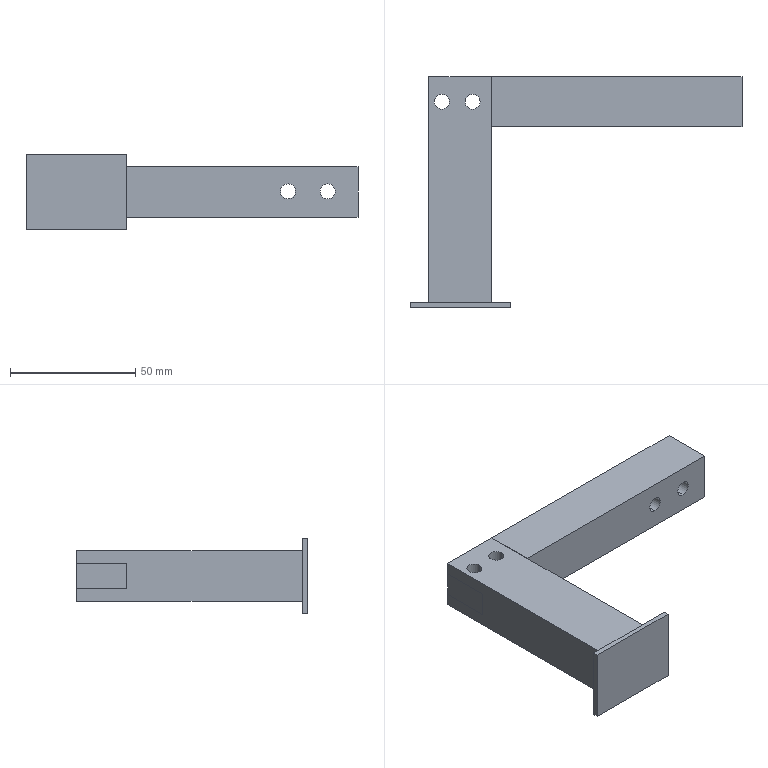Part | SolidWorks | features Cut 3, ICE 2, Extrusion 1 | 2 solids | 41 faces | box 132.5 x 92 x 30 mm | volume 85138 mm3 | plane 25 | cylinder 16 | commonest cylinder face diameters 6 x16
STEP:
#1=CARTESIAN_POINT('',(-15.29,82.,4.756));
#2=VERTEX_POINT('',#1);
#3=CARTESIAN_POINT('',(-9.29,82.,4.756));
#4=VERTEX_POINT('',#3);
#5=CARTESIAN_POINT('',(-12.29,82.,4.756));
#6=DIRECTION('',(0.,0.,1.));
#7=DIRECTION('',(1.,0.,0.));
#8=AXIS2_PLACEMENT_3D('',#5,#6,#7);
#9=CIRCLE('',#8,3.);
#10=EDGE_CURVE('',#2,#4,#9,.T.);
#11=ORIENTED_EDGE('',*,*,#10,.F.);
#12=CARTESIAN_POINT('',(-15.29,82.,9.756));
#13=VERTEX_POINT('',#12);
#14=CARTESIAN_POINT('',(-15.29,82.,-19.244));
#15=DIRECTION('',(0.,0.,1.));
#16=VECTOR('',#15,1000.);
#17=LINE('',#14,#16);
#18=EDGE_CURVE('',#2,#13,#17,.T.);
#19=ORIENTED_EDGE('',*,*,#18,.T.);
#20=CARTESIAN_POINT('',(-9.29,82.,9.756));
#21=VERTEX_POINT('',#20);
#22=CARTESIAN_POINT('',(-12.29,82.,9.756));
#23=DIRECTION('',(0.,0.,1.));
#24=DIRECTION('',(1.,0.,0.));
#25=AXIS2_PLACEMENT_3D('',#22,#23,#24);
#26=CIRCLE('',#25,3.);
#27=EDGE_CURVE('',#13,#21,#26,.T.);
#28=ORIENTED_EDGE('',*,*,#27,.T.);
#29=CARTESIAN_POINT('',(-9.29,82.,-19.244));
#30=DIRECTION('',(0.,0.,1.));
#31=VECTOR('',#30,1000.);
#32=LINE('',#29,#31);
#33=EDGE_CURVE('',#4,#21,#32,.T.);
#34=ORIENTED_EDGE('',*,*,#33,.F.);
#35=EDGE_LOOP('',(#11,#19,#28,#34));
#36=FACE_OUTER_BOUND('',#35,.T.);
#37=CARTESIAN_POINT('',(-12.29,82.,-19.244));
#38=DIRECTION('',(0.,0.,1.));
#39=DIRECTION('',(1.,0.,0.));
#40=AXIS2_PLACEMENT_3D('',#37,#38,#39);
#41=CYLINDRICAL_SURFACE('',#40,3.);
#42=ADVANCED_FACE('',(#36),#41,.F.);
#43=CARTESIAN_POINT('',(-3.,82.,4.756));
#44=VERTEX_POINT('',#43);
#45=CARTESIAN_POINT('',(3.,82.,4.756));
#46=VERTEX_POINT('',#45);
#47=CARTESIAN_POINT('',(0.,82.,4.756));
#48=DIRECTION('',(0.,0.,1.));
#49=DIRECTION('',(1.,0.,0.));
#50=AXIS2_PLACEMENT_3D('',#47,#48,#49);
#51=CIRCLE('',#50,3.);
#52=EDGE_CURVE('',#44,#46,#51,.T.);
#53=ORIENTED_EDGE('',*,*,#52,.F.);
#54=CARTESIAN_POINT('',(-3.,82.,9.756));
#55=VERTEX_POINT('',#54);
#56=CARTESIAN_POINT('',(-3.,82.,-19.244));
#57=DIRECTION('',(0.,0.,1.));
#58=VECTOR('',#57,1000.);
#59=LINE('',#56,#58);
#60=EDGE_CURVE('',#44,#55,#59,.T.);
#61=ORIENTED_EDGE('',*,*,#60,.T.);
#62=CARTESIAN_POINT('',(3.,82.,9.756));
#63=VERTEX_POINT('',#62);
#64=CARTESIAN_POINT('',(0.,82.,9.756));
#65=DIRECTION('',(0.,0.,1.));
#66=DIRECTION('',(1.,0.,0.));
#67=AXIS2_PLACEMENT_3D('',#64,#65,#66);
#68=CIRCLE('',#67,3.);
#69=EDGE_CURVE('',#55,#63,#68,.T.);
#70=ORIENTED_EDGE('',*,*,#69,.T.);
#71=CARTESIAN_POINT('',(3.,82.,-19.244));
#72=DIRECTION('',(0.,0.,1.));
#73=VECTOR('',#72,1000.);
#74=LINE('',#71,#73);
#75=EDGE_CURVE('',#46,#63,#74,.T.);
#76=ORIENTED_EDGE('',*,*,#75,.F.);
#77=EDGE_LOOP('',(#53,#61,#70,#76));
#78=FACE_OUTER_BOUND('',#77,.T.);
#79=CARTESIAN_POINT('',(0.,82.,-19.244));
#80=DIRECTION('',(0.,0.,1.));
#81=DIRECTION('',(1.,0.,0.));
#82=AXIS2_PLACEMENT_3D('',#79,#80,#81);
#83=CYLINDRICAL_SURFACE('',#82,3.);
#84=ADVANCED_FACE('',(#78),#83,.F.);
#85=CARTESIAN_POINT('',(-15.29,82.,-10.244));
#86=VERTEX_POINT('',#85);
#87=CARTESIAN_POINT('',(-9.29,82.,-10.244));
#88=VERTEX_POINT('',#87);
#89=CARTESIAN_POINT('',(-12.29,82.,-10.244));
#90=DIRECTION('',(0.,0.,1.));
#91=DIRECTION('',(1.,0.,0.));
#92=AXIS2_PLACEMENT_3D('',#89,#90,#91);
#93=CIRCLE('',#92,3.);
#94=EDGE_CURVE('',#86,#88,#93,.T.);
#95=ORIENTED_EDGE('',*,*,#94,.F.);
#96=CARTESIAN_POINT('',(-15.29,82.,-5.244));
#97=VERTEX_POINT('',#96);
#98=CARTESIAN_POINT('',(-15.29,82.,-19.244));
#99=DIRECTION('',(0.,0.,1.));
#100=VECTOR('',#99,1000.);
#101=LINE('',#98,#100);
#102=EDGE_CURVE('',#86,#97,#101,.T.);
#103=ORIENTED_EDGE('',*,*,#102,.T.);
#104=CARTESIAN_POINT('',(-9.29,82.,-5.244));
#105=VERTEX_POINT('',#104);
#106=CARTESIAN_POINT('',(-12.29,82.,-5.244));
#107=DIRECTION('',(0.,0.,-1.));
#108=DIRECTION('',(-1.,0.,0.));
#109=AXIS2_PLACEMENT_3D('',#106,#107,#108);
#110=CIRCLE('',#109,3.);
#111=EDGE_CURVE('',#105,#97,#110,.T.);
#112=ORIENTED_EDGE('',*,*,#111,.F.);
#113=CARTESIAN_POINT('',(-9.29,82.,-19.244));
#114=DIRECTION('',(0.,0.,1.));
#115=VECTOR('',#114,1000.);
#116=LINE('',#113,#115);
#117=EDGE_CURVE('',#88,#105,#116,.T.);
#118=ORIENTED_EDGE('',*,*,#117,.F.);
#119=EDGE_LOOP('',(#95,#103,#112,#118));
#120=FACE_OUTER_BOUND('',#119,.T.);
#121=CARTESIAN_POINT('',(-12.29,82.,-19.244));
#122=DIRECTION('',(0.,0.,1.));
#123=DIRECTION('',(1.,0.,0.));
#124=AXIS2_PLACEMENT_3D('',#121,#122,#123);
#125=CYLINDRICAL_SURFACE('',#124,3.);
#126=ADVANCED_FACE('',(#120),#125,.F.);
#127=CARTESIAN_POINT('',(-3.,82.,-10.244));
#128=VERTEX_POINT('',#127);
#129=CARTESIAN_POINT('',(3.,82.,-10.244));
#130=VERTEX_POINT('',#129);
#131=CARTESIAN_POINT('',(0.,82.,-10.244));
#132=DIRECTION('',(0.,0.,1.));
#133=DIRECTION('',(1.,0.,0.));
#134=AXIS2_PLACEMENT_3D('',#131,#132,#133);
#135=CIRCLE('',#134,3.);
#136=EDGE_CURVE('',#128,#130,#135,.T.);
#137=ORIENTED_EDGE('',*,*,#136,.F.);
#138=CARTESIAN_POINT('',(-3.,82.,-5.244));
#139=VERTEX_POINT('',#138);
#140=CARTESIAN_POINT('',(-3.,82.,-19.244));
#141=DIRECTION('',(0.,0.,1.));
#142=VECTOR('',#141,1000.);
#143=LINE('',#140,#142);
#144=EDGE_CURVE('',#128,#139,#143,.T.);
#145=ORIENTED_EDGE('',*,*,#144,.T.);
#146=CARTESIAN_POINT('',(3.,82.,-5.244));
#147=VERTEX_POINT('',#146);
#148=CARTESIAN_POINT('',(0.,82.,-5.244));
#149=DIRECTION('',(0.,0.,-1.));
#150=DIRECTION('',(-1.,0.,0.));
#151=AXIS2_PLACEMENT_3D('',#148,#149,#150);
#152=CIRCLE('',#151,3.);
#153=EDGE_CURVE('',#147,#139,#152,.T.);
#154=ORIENTED_EDGE('',*,*,#153,.F.);
#155=CARTESIAN_POINT('',(3.,82.,-19.244));
#156=DIRECTION('',(0.,0.,1.));
#157=VECTOR('',#156,1000.);
#158=LINE('',#155,#157);
#159=EDGE_CURVE('',#130,#147,#158,.T.);
#160=ORIENTED_EDGE('',*,*,#159,.F.);
#161=EDGE_LOOP('',(#137,#145,#154,#160));
#162=FACE_OUTER_BOUND('',#161,.T.);
#163=CARTESIAN_POINT('',(0.,82.,-19.244));
#164=DIRECTION('',(0.,0.,1.));
#165=DIRECTION('',(1.,0.,0.));
#166=AXIS2_PLACEMENT_3D('',#163,#164,#165);
#167=CYLINDRICAL_SURFACE('',#166,3.);
#168=ADVANCED_FACE('',(#162),#167,.F.);
#169=CARTESIAN_POINT('',(-17.5,92.,4.756));
#170=VERTEX_POINT('',#169);
#171=CARTESIAN_POINT('',(7.5,92.,4.756));
#172=VERTEX_POINT('',#171);
#173=CARTESIAN_POINT('',(-17.5,92.,4.756));
#174=DIRECTION('',(1.,0.,0.));
#175=VECTOR('',#174,1000.);
#176=LINE('',#173,#175);
#177=EDGE_CURVE('',#170,#172,#176,.T.);
#178=ORIENTED_EDGE('',*,*,#177,.F.);
#179=CARTESIAN_POINT('',(-17.5,92.,9.756));
#180=VERTEX_POINT('',#179);
#181=CARTESIAN_POINT('',(-17.5,92.,-10.244));
#182=DIRECTION('',(0.,0.,1.));
#183=VECTOR('',#182,1000.);
#184=LINE('',#181,#183);
#185=EDGE_CURVE('',#170,#180,#184,.T.);
#186=ORIENTED_EDGE('',*,*,#185,.T.);
#187=CARTESIAN_POINT('',(7.5,92.,9.756));
#188=VERTEX_POINT('',#187);
#189=CARTESIAN_POINT('',(-17.5,92.,9.756));
#190=DIRECTION('',(1.,0.,0.));
#191=VECTOR('',#190,1000.);
#192=LINE('',#189,#191);
#193=EDGE_CURVE('',#180,#188,#192,.T.);
#194=ORIENTED_EDGE('',*,*,#193,.T.);
#195=CARTESIAN_POINT('',(7.5,92.,-10.244));
#196=DIRECTION('',(0.,0.,-1.));
#197=VECTOR('',#196,1000.);
#198=LINE('',#195,#197);
#199=EDGE_CURVE('',#188,#172,#198,.T.);
#200=ORIENTED_EDGE('',*,*,#199,.T.);
#201=EDGE_LOOP('',(#178,#186,#194,#200));
#202=FACE_OUTER_BOUND('',#201,.T.);
#203=CARTESIAN_POINT('',(0.,92.,0.));
#204=DIRECTION('',(0.,1.,0.));
#205=DIRECTION('',(0.,0.,1.));
#206=AXIS2_PLACEMENT_3D('',#203,#204,#205);
#207=PLANE('',#206);
#208=ADVANCED_FACE('',(#202),#207,.T.);
#209=CARTESIAN_POINT('',(15.,0.,14.756));
#210=VERTEX_POINT('',#209);
#211=CARTESIAN_POINT('',(15.,0.,-15.244));
#212=VERTEX_POINT('',#211);
#213=CARTESIAN_POINT('',(15.,0.,-15.244));
#214=DIRECTION('',(0.,0.,-1.));
#215=VECTOR('',#214,1000.);
#216=LINE('',#213,#215);
#217=EDGE_CURVE('',#210,#212,#216,.T.);
#218=ORIENTED_EDGE('',*,*,#217,.T.);
#219=CARTESIAN_POINT('',(15.,2.,-15.244));
#220=VERTEX_POINT('',#219);
#221=CARTESIAN_POINT('',(15.,2.,-15.244));
#222=DIRECTION('',(0.,-1.,0.));
#223=VECTOR('',#222,1000.);
#224=LINE('',#221,#223);
#225=EDGE_CURVE('',#220,#212,#224,.T.);
#226=ORIENTED_EDGE('',*,*,#225,.F.);
#227=CARTESIAN_POINT('',(15.,2.,14.756));
#228=VERTEX_POINT('',#227);
#229=CARTESIAN_POINT('',(15.,2.,-15.244));
#230=DIRECTION('',(0.,0.,-1.));
#231=VECTOR('',#230,1000.);
#232=LINE('',#229,#231);
#233=EDGE_CURVE('',#228,#220,#232,.T.);
#234=ORIENTED_EDGE('',*,*,#233,.F.);
#235=CARTESIAN_POINT('',(15.,2.,14.756));
#236=DIRECTION('',(0.,-1.,0.));
#237=VECTOR('',#236,1000.);
#238=LINE('',#235,#237);
#239=EDGE_CURVE('',#228,#210,#238,.T.);
#240=ORIENTED_EDGE('',*,*,#239,.T.);
#241=EDGE_LOOP('',(#218,#226,#234,#240));
#242=FACE_OUTER_BOUND('',#241,.T.);
#243=CARTESIAN_POINT('',(15.,2.,-15.244));
#244=DIRECTION('',(-1.,0.,0.));
#245=DIRECTION('',(0.,0.,1.));
#246=AXIS2_PLACEMENT_3D('',#243,#244,#245);
#247=PLANE('',#246);
#248=ADVANCED_FACE('',(#242),#247,.F.);
#249=CARTESIAN_POINT('',(-25.,0.,-15.244));
#250=VERTEX_POINT('',#249);
#251=CARTESIAN_POINT('',(-25.,0.,-15.244));
#252=DIRECTION('',(-1.,0.,0.));
#253=VECTOR('',#252,1000.);
#254=LINE('',#251,#253);
#255=EDGE_CURVE('',#212,#250,#254,.T.);
#256=ORIENTED_EDGE('',*,*,#255,.T.);
#257=CARTESIAN_POINT('',(-25.,2.,-15.244));
#258=VERTEX_POINT('',#257);
#259=CARTESIAN_POINT('',(-25.,2.,-15.244));
#260=DIRECTION('',(0.,-1.,0.));
#261=VECTOR('',#260,1000.);
#262=LINE('',#259,#261);
#263=EDGE_CURVE('',#258,#250,#262,.T.);
#264=ORIENTED_EDGE('',*,*,#263,.F.);
#265=CARTESIAN_POINT('',(-25.,2.,-15.244));
#266=DIRECTION('',(-1.,0.,0.));
#267=VECTOR('',#266,1000.);
#268=LINE('',#265,#267);
#269=EDGE_CURVE('',#220,#258,#268,.T.);
#270=ORIENTED_EDGE('',*,*,#269,.F.);
#271=ORIENTED_EDGE('',*,*,#225,.T.);
#272=EDGE_LOOP('',(#256,#264,#270,#271));
#273=FACE_OUTER_BOUND('',#272,.T.);
#274=CARTESIAN_POINT('',(-25.,2.,-15.244));
#275=DIRECTION('',(0.,0.,1.));
#276=DIRECTION('',(1.,0.,0.));
#277=AXIS2_PLACEMENT_3D('',#274,#275,#276);
#278=PLANE('',#277);
#279=ADVANCED_FACE('',(#273),#278,.F.);
#280=CARTESIAN_POINT('',(-25.,0.,14.756));
#281=VERTEX_POINT('',#280);
#282=CARTESIAN_POINT('',(-25.,0.,-15.244));
#283=DIRECTION('',(0.,0.,1.));
#284=VECTOR('',#283,1000.);
#285=LINE('',#282,#284);
#286=EDGE_CURVE('',#250,#281,#285,.T.);
#287=ORIENTED_EDGE('',*,*,#286,.T.);
#288=CARTESIAN_POINT('',(-25.,2.,14.756));
#289=VERTEX_POINT('',#288);
#290=CARTESIAN_POINT('',(-25.,2.,14.756));
#291=DIRECTION('',(0.,-1.,0.));
#292=VECTOR('',#291,1000.);
#293=LINE('',#290,#292);
#294=EDGE_CURVE('',#289,#281,#293,.T.);
#295=ORIENTED_EDGE('',*,*,#294,.F.);
#296=CARTESIAN_POINT('',(-25.,2.,-15.244));
#297=DIRECTION('',(0.,0.,1.));
#298=VECTOR('',#297,1000.);
#299=LINE('',#296,#298);
#300=EDGE_CURVE('',#258,#289,#299,.T.);
#301=ORIENTED_EDGE('',*,*,#300,.F.);
#302=ORIENTED_EDGE('',*,*,#263,.T.);
#303=EDGE_LOOP('',(#287,#295,#301,#302));
#304=FACE_OUTER_BOUND('',#303,.T.);
#305=CARTESIAN_POINT('',(-25.,2.,-15.244));
#306=DIRECTION('',(1.,0.,0.));
#307=DIRECTION('',(0.,0.,-1.));
#308=AXIS2_PLACEMENT_3D('',#305,#306,#307);
#309=PLANE('',#308);
#310=ADVANCED_FACE('',(#304),#309,.F.);
#311=CARTESIAN_POINT('',(-25.,0.,14.756));
#312=DIRECTION('',(1.,0.,0.));
#313=VECTOR('',#312,1000.);
#314=LINE('',#311,#313);
#315=EDGE_CURVE('',#281,#210,#314,.T.);
#316=ORIENTED_EDGE('',*,*,#315,.T.);
#317=ORIENTED_EDGE('',*,*,#239,.F.);
#318=CARTESIAN_POINT('',(-25.,2.,14.756));
#319=DIRECTION('',(1.,0.,0.));
#320=VECTOR('',#319,1000.);
#321=LINE('',#318,#320);
#322=EDGE_CURVE('',#289,#228,#321,.T.);
#323=ORIENTED_EDGE('',*,*,#322,.F.);
#324=ORIENTED_EDGE('',*,*,#294,.T.);
#325=EDGE_LOOP('',(#316,#317,#323,#324));
#326=FACE_OUTER_BOUND('',#325,.T.);
#327=CARTESIAN_POINT('',(-25.,2.,14.756));
#328=DIRECTION('',(0.,0.,-1.));
#329=DIRECTION('',(-1.,0.,0.));
#330=AXIS2_PLACEMENT_3D('',#327,#328,#329);
#331=PLANE('',#330);
#332=ADVANCED_FACE('',(#326),#331,.F.);
#333=CARTESIAN_POINT('',(7.5,2.,9.756));
#334=VERTEX_POINT('',#333);
#335=CARTESIAN_POINT('',(7.5,2.,-10.244));
#336=VERTEX_POINT('',#335);
#337=CARTESIAN_POINT('',(7.5,2.,-10.244));
#338=DIRECTION('',(0.,0.,-1.));
#339=VECTOR('',#338,1000.);
#340=LINE('',#337,#339);
#341=EDGE_CURVE('',#334,#336,#340,.T.);
#342=ORIENTED_EDGE('',*,*,#341,.F.);
#343=CARTESIAN_POINT('',(-17.5,2.,9.756));
#344=VERTEX_POINT('',#343);
#345=CARTESIAN_POINT('',(-17.5,2.,9.756));
#346=DIRECTION('',(1.,0.,0.));
#347=VECTOR('',#346,1000.);
#348=LINE('',#345,#347);
#349=EDGE_CURVE('',#344,#334,#348,.T.);
#350=ORIENTED_EDGE('',*,*,#349,.F.);
#351=CARTESIAN_POINT('',(-17.5,2.,-10.244));
#352=VERTEX_POINT('',#351);
#353=CARTESIAN_POINT('',(-17.5,2.,-10.244));
#354=DIRECTION('',(0.,0.,1.));
#355=VECTOR('',#354,1000.);
#356=LINE('',#353,#355);
#357=EDGE_CURVE('',#352,#344,#356,.T.);
#358=ORIENTED_EDGE('',*,*,#357,.F.);
#359=CARTESIAN_POINT('',(-17.5,2.,-10.244));
#360=DIRECTION('',(-1.,0.,0.));
#361=VECTOR('',#360,1000.);
#362=LINE('',#359,#361);
#363=EDGE_CURVE('',#336,#352,#362,.T.);
#364=ORIENTED_EDGE('',*,*,#363,.F.);
#365=EDGE_LOOP('',(#342,#350,#358,#364));
#366=FACE_BOUND('',#365,.T.);
#367=ORIENTED_EDGE('',*,*,#233,.T.);
#368=ORIENTED_EDGE('',*,*,#269,.T.);
#369=ORIENTED_EDGE('',*,*,#300,.T.);
#370=ORIENTED_EDGE('',*,*,#322,.T.);
#371=EDGE_LOOP('',(#367,#368,#369,#370));
#372=FACE_OUTER_BOUND('',#371,.T.);
#373=CARTESIAN_POINT('',(0.,2.,0.));
#374=DIRECTION('',(0.,1.,0.));
#375=DIRECTION('',(0.,0.,1.));
#376=AXIS2_PLACEMENT_3D('',#373,#374,#375);
#377=PLANE('',#376);
#378=ADVANCED_FACE('',(#366,#372),#377,.T.);
#379=ORIENTED_EDGE('',*,*,#217,.F.);
#380=ORIENTED_EDGE('',*,*,#315,.F.);
#381=ORIENTED_EDGE('',*,*,#286,.F.);
#382=ORIENTED_EDGE('',*,*,#255,.F.);
#383=EDGE_LOOP('',(#379,#380,#381,#382));
#384=FACE_OUTER_BOUND('',#383,.T.);
#385=CARTESIAN_POINT('',(0.,0.,0.));
#386=DIRECTION('',(0.,1.,0.));
#387=DIRECTION('',(0.,0.,1.));
#388=AXIS2_PLACEMENT_3D('',#385,#386,#387);
#389=PLANE('',#388);
#390=ADVANCED_FACE('',(#384),#389,.F.);
#391=CARTESIAN_POINT('',(7.5,72.,4.756));
#392=VERTEX_POINT('',#391);
#393=CARTESIAN_POINT('',(7.5,72.,-5.244));
#394=VERTEX_POINT('',#393);
#395=CARTESIAN_POINT('',(7.5,72.,-5.244));
#396=DIRECTION('',(0.,0.,-1.));
#397=VECTOR('',#396,1000.);
#398=LINE('',#395,#397);
#399=EDGE_CURVE('',#392,#394,#398,.T.);
#400=ORIENTED_EDGE('',*,*,#399,.F.);
#401=CARTESIAN_POINT('',(7.5,72.,4.756));
#402=DIRECTION('',(0.,1.,0.));
#403=VECTOR('',#402,1000.);
#404=LINE('',#401,#403);
#405=EDGE_CURVE('',#392,#172,#404,.T.);
#406=ORIENTED_EDGE('',*,*,#405,.T.);
#407=ORIENTED_EDGE('',*,*,#199,.F.);
#408=CARTESIAN_POINT('',(7.5,92.,9.756));
#409=DIRECTION('',(0.,-1.,0.));
#410=VECTOR('',#409,1000.);
#411=LINE('',#408,#410);
#412=EDGE_CURVE('',#188,#334,#411,.T.);
#413=ORIENTED_EDGE('',*,*,#412,.T.);
#414=ORIENTED_EDGE('',*,*,#341,.T.);
#415=CARTESIAN_POINT('',(7.5,92.,-10.244));
#416=VERTEX_POINT('',#415);
#417=CARTESIAN_POINT('',(7.5,92.,-10.244));
#418=DIRECTION('',(0.,-1.,0.));
#419=VECTOR('',#418,1000.);
#420=LINE('',#417,#419);
#421=EDGE_CURVE('',#416,#336,#420,.T.);
#422=ORIENTED_EDGE('',*,*,#421,.F.);
#423=CARTESIAN_POINT('',(7.5,92.,-5.244));
#424=VERTEX_POINT('',#423);
#425=CARTESIAN_POINT('',(7.5,92.,-10.244));
#426=DIRECTION('',(0.,0.,-1.));
#427=VECTOR('',#426,1000.);
#428=LINE('',#425,#427);
#429=EDGE_CURVE('',#424,#416,#428,.T.);
#430=ORIENTED_EDGE('',*,*,#429,.F.);
#431=CARTESIAN_POINT('',(7.5,72.,-5.244));
#432=DIRECTION('',(0.,1.,0.));
#433=VECTOR('',#432,1000.);
#434=LINE('',#431,#433);
#435=EDGE_CURVE('',#394,#424,#434,.T.);
#436=ORIENTED_EDGE('',*,*,#435,.F.);
#437=EDGE_LOOP('',(#400,#406,#407,#413,#414,#422,#430,#436));
#438=FACE_OUTER_BOUND('',#437,.T.);
#439=CARTESIAN_POINT('',(7.5,92.,-10.244));
#440=DIRECTION('',(-1.,0.,0.));
#441=DIRECTION('',(0.,0.,1.));
#442=AXIS2_PLACEMENT_3D('',#439,#440,#441);
#443=PLANE('',#442);
#444=ADVANCED_FACE('',(#438),#443,.F.);
#445=CARTESIAN_POINT('',(-12.29,82.,-10.244));
#446=DIRECTION('',(0.,0.,1.));
#447=DIRECTION('',(1.,0.,0.));
#448=AXIS2_PLACEMENT_3D('',#445,#446,#447);
#449=CIRCLE('',#448,3.);
#450=EDGE_CURVE('',#88,#86,#449,.T.);
#451=ORIENTED_EDGE('',*,*,#450,.T.);
#452=ORIENTED_EDGE('',*,*,#94,.T.);
#453=EDGE_LOOP('',(#451,#452));
#454=FACE_BOUND('',#453,.T.);
#455=CARTESIAN_POINT('',(0.,82.,-10.244));
#456=DIRECTION('',(0.,0.,1.));
#457=DIRECTION('',(1.,0.,0.));
#458=AXIS2_PLACEMENT_3D('',#455,#456,#457);
#459=CIRCLE('',#458,3.);
#460=EDGE_CURVE('',#130,#128,#459,.T.);
#461=ORIENTED_EDGE('',*,*,#460,.T.);
#462=ORIENTED_EDGE('',*,*,#136,.T.);
#463=EDGE_LOOP('',(#461,#462));
#464=FACE_BOUND('',#463,.T.);
#465=ORIENTED_EDGE('',*,*,#363,.T.);
#466=CARTESIAN_POINT('',(-17.5,92.,-10.244));
#467=VERTEX_POINT('',#466);
#468=CARTESIAN_POINT('',(-17.5,92.,-10.244));
#469=DIRECTION('',(0.,-1.,0.));
#470=VECTOR('',#469,1000.);
#471=LINE('',#468,#470);
#472=EDGE_CURVE('',#467,#352,#471,.T.);
#473=ORIENTED_EDGE('',*,*,#472,.F.);
#474=CARTESIAN_POINT('',(-17.5,92.,-10.244));
#475=DIRECTION('',(-1.,0.,0.));
#476=VECTOR('',#475,1000.);
#477=LINE('',#474,#476);
#478=EDGE_CURVE('',#416,#467,#477,.T.);
#479=ORIENTED_EDGE('',*,*,#478,.F.);
#480=ORIENTED_EDGE('',*,*,#421,.T.);
#481=EDGE_LOOP('',(#465,#473,#479,#480));
#482=FACE_OUTER_BOUND('',#481,.T.);
#483=CARTESIAN_POINT('',(-17.5,92.,-10.244));
#484=DIRECTION('',(0.,0.,1.));
#485=DIRECTION('',(1.,0.,0.));
#486=AXIS2_PLACEMENT_3D('',#483,#484,#485);
#487=PLANE('',#486);
#488=ADVANCED_FACE('',(#454,#464,#482),#487,.F.);
#489=ORIENTED_EDGE('',*,*,#185,.F.);
#490=CARTESIAN_POINT('',(-17.5,72.,4.756));
#491=VERTEX_POINT('',#490);
#492=CARTESIAN_POINT('',(-17.5,72.,4.756));
#493=DIRECTION('',(0.,1.,0.));
#494=VECTOR('',#493,1000.);
#495=LINE('',#492,#494);
#496=EDGE_CURVE('',#491,#170,#495,.T.);
#497=ORIENTED_EDGE('',*,*,#496,.F.);
#498=CARTESIAN_POINT('',(-17.5,72.,-5.244));
#499=VERTEX_POINT('',#498);
#500=CARTESIAN_POINT('',(-17.5,72.,-5.244));
#501=DIRECTION('',(0.,0.,1.));
#502=VECTOR('',#501,1000.);
#503=LINE('',#500,#502);
#504=EDGE_CURVE('',#499,#491,#503,.T.);
#505=ORIENTED_EDGE('',*,*,#504,.F.);
#506=CARTESIAN_POINT('',(-17.5,92.,-5.244));
#507=VERTEX_POINT('',#506);
#508=CARTESIAN_POINT('',(-17.5,72.,-5.244));
#509=DIRECTION('',(0.,1.,0.));
#510=VECTOR('',#509,1000.);
#511=LINE('',#508,#510);
#512=EDGE_CURVE('',#499,#507,#511,.T.);
#513=ORIENTED_EDGE('',*,*,#512,.T.);
#514=CARTESIAN_POINT('',(-17.5,92.,-10.244));
#515=DIRECTION('',(0.,0.,1.));
#516=VECTOR('',#515,1000.);
#517=LINE('',#514,#516);
#518=EDGE_CURVE('',#467,#507,#517,.T.);
#519=ORIENTED_EDGE('',*,*,#518,.F.);
#520=ORIENTED_EDGE('',*,*,#472,.T.);
#521=ORIENTED_EDGE('',*,*,#357,.T.);
#522=CARTESIAN_POINT('',(-17.5,92.,9.756));
#523=DIRECTION('',(0.,-1.,0.));
#524=VECTOR('',#523,1000.);
#525=LINE('',#522,#524);
#526=EDGE_CURVE('',#180,#344,#525,.T.);
#527=ORIENTED_EDGE('',*,*,#526,.F.);
#528=EDGE_LOOP('',(#489,#497,#505,#513,#519,#520,#521,#527));
#529=FACE_OUTER_BOUND('',#528,.T.);
#530=CARTESIAN_POINT('',(-17.5,92.,-10.244));
#531=DIRECTION('',(1.,0.,0.));
#532=DIRECTION('',(0.,0.,-1.));
#533=AXIS2_PLACEMENT_3D('',#530,#531,#532);
#534=PLANE('',#533);
#535=ADVANCED_FACE('',(#529),#534,.F.);
#536=CARTESIAN_POINT('',(-12.29,82.,9.756));
#537=DIRECTION('',(0.,0.,1.));
#538=DIRECTION('',(1.,0.,0.));
#539=AXIS2_PLACEMENT_3D('',#536,#537,#538);
#540=CIRCLE('',#539,3.);
#541=EDGE_CURVE('',#21,#13,#540,.T.);
#542=ORIENTED_EDGE('',*,*,#541,.F.);
#543=ORIENTED_EDGE('',*,*,#27,.F.);
#544=EDGE_LOOP('',(#542,#543));
#545=FACE_BOUND('',#544,.T.);
#546=CARTESIAN_POINT('',(0.,82.,9.756));
#547=DIRECTION('',(0.,0.,1.));
#548=DIRECTION('',(1.,0.,0.));
#549=AXIS2_PLACEMENT_3D('',#546,#547,#548);
#550=CIRCLE('',#549,3.);
#551=EDGE_CURVE('',#63,#55,#550,.T.);
#552=ORIENTED_EDGE('',*,*,#551,.F.);
#553=ORIENTED_EDGE('',*,*,#69,.F.);
#554=EDGE_LOOP('',(#552,#553));
#555=FACE_BOUND('',#554,.T.);
#556=ORIENTED_EDGE('',*,*,#349,.T.);
#557=ORIENTED_EDGE('',*,*,#412,.F.);
#558=ORIENTED_EDGE('',*,*,#193,.F.);
#559=ORIENTED_EDGE('',*,*,#526,.T.);
#560=EDGE_LOOP('',(#556,#557,#558,#559));
#561=FACE_OUTER_BOUND('',#560,.T.);
#562=CARTESIAN_POINT('',(-17.5,92.,9.756));
#563=DIRECTION('',(0.,0.,-1.));
#564=DIRECTION('',(-1.,0.,0.));
#565=AXIS2_PLACEMENT_3D('',#562,#563,#564);
#566=PLANE('',#565);
#567=ADVANCED_FACE('',(#545,#555,#561),#566,.F.);
#568=CARTESIAN_POINT('',(-17.5,92.,-5.244));
#569=DIRECTION('',(-1.,0.,0.));
#570=VECTOR('',#569,1000.);
#571=LINE('',#568,#570);
#572=EDGE_CURVE('',#424,#507,#571,.T.);
#573=ORIENTED_EDGE('',*,*,#572,.F.);
#574=ORIENTED_EDGE('',*,*,#429,.T.);
#575=ORIENTED_EDGE('',*,*,#478,.T.);
#576=ORIENTED_EDGE('',*,*,#518,.T.);
#577=EDGE_LOOP('',(#573,#574,#575,#576));
#578=FACE_OUTER_BOUND('',#577,.T.);
#579=CARTESIAN_POINT('',(0.,92.,0.));
#580=DIRECTION('',(0.,1.,0.));
#581=DIRECTION('',(0.,0.,1.));
#582=AXIS2_PLACEMENT_3D('',#579,#580,#581);
#583=PLANE('',#582);
#584=ADVANCED_FACE('',(#578),#583,.T.);
#585=CARTESIAN_POINT('',(-12.29,82.,4.756));
#586=DIRECTION('',(0.,0.,1.));
#587=DIRECTION('',(1.,0.,0.));
#588=AXIS2_PLACEMENT_3D('',#585,#586,#587);
#589=CIRCLE('',#588,3.);
#590=EDGE_CURVE('',#4,#2,#589,.T.);
#591=ORIENTED_EDGE('',*,*,#590,.T.);
#592=ORIENTED_EDGE('',*,*,#10,.T.);
#593=EDGE_LOOP('',(#591,#592));
#594=FACE_BOUND('',#593,.T.);
#595=CARTESIAN_POINT('',(0.,82.,4.756));
#596=DIRECTION('',(0.,0.,1.));
#597=DIRECTION('',(1.,0.,0.));
#598=AXIS2_PLACEMENT_3D('',#595,#596,#597);
#599=CIRCLE('',#598,3.);
#600=EDGE_CURVE('',#46,#44,#599,.T.);
#601=ORIENTED_EDGE('',*,*,#600,.T.);
#602=ORIENTED_EDGE('',*,*,#52,.T.);
#603=EDGE_LOOP('',(#601,#602));
#604=FACE_BOUND('',#603,.T.);
#605=ORIENTED_EDGE('',*,*,#177,.T.);
#606=ORIENTED_EDGE('',*,*,#405,.F.);
#607=CARTESIAN_POINT('',(-17.5,72.,4.756));
#608=DIRECTION('',(1.,0.,0.));
#609=VECTOR('',#608,1000.);
#610=LINE('',#607,#609);
#611=EDGE_CURVE('',#491,#392,#610,.T.);
#612=ORIENTED_EDGE('',*,*,#611,.F.);
#613=ORIENTED_EDGE('',*,*,#496,.T.);
#614=EDGE_LOOP('',(#605,#606,#612,#613));
#615=FACE_OUTER_BOUND('',#614,.T.);
#616=CARTESIAN_POINT('',(-17.5,72.,4.756));
#617=DIRECTION('',(0.,0.,1.));
#618=DIRECTION('',(1.,0.,0.));
#619=AXIS2_PLACEMENT_3D('',#616,#617,#618);
#620=PLANE('',#619);
#621=ADVANCED_FACE('',(#594,#604,#615),#620,.F.);
#622=ORIENTED_EDGE('',*,*,#111,.T.);
#623=CARTESIAN_POINT('',(-12.29,82.,-5.244));
#624=DIRECTION('',(0.,0.,-1.));
#625=DIRECTION('',(-1.,0.,0.));
#626=AXIS2_PLACEMENT_3D('',#623,#624,#625);
#627=CIRCLE('',#626,3.);
#628=EDGE_CURVE('',#97,#105,#627,.T.);
#629=ORIENTED_EDGE('',*,*,#628,.T.);
#630=EDGE_LOOP('',(#622,#629));
#631=FACE_BOUND('',#630,.T.);
#632=ORIENTED_EDGE('',*,*,#153,.T.);
#633=CARTESIAN_POINT('',(0.,82.,-5.244));
#634=DIRECTION('',(0.,0.,-1.));
#635=DIRECTION('',(-1.,0.,0.));
#636=AXIS2_PLACEMENT_3D('',#633,#634,#635);
#637=CIRCLE('',#636,3.);
#638=EDGE_CURVE('',#139,#147,#637,.T.);
#639=ORIENTED_EDGE('',*,*,#638,.T.);
#640=EDGE_LOOP('',(#632,#639));
#641=FACE_BOUND('',#640,.T.);
#642=ORIENTED_EDGE('',*,*,#572,.T.);
#643=ORIENTED_EDGE('',*,*,#512,.F.);
#644=CARTESIAN_POINT('',(-17.5,72.,-5.244));
#645=DIRECTION('',(-1.,0.,0.));
#646=VECTOR('',#645,1000.);
#647=LINE('',#644,#646);
#648=EDGE_CURVE('',#394,#499,#647,.T.);
#649=ORIENTED_EDGE('',*,*,#648,.F.);
#650=ORIENTED_EDGE('',*,*,#435,.T.);
#651=EDGE_LOOP('',(#642,#643,#649,#650));
#652=FACE_OUTER_BOUND('',#651,.T.);
#653=CARTESIAN_POINT('',(-17.5,72.,-5.244));
#654=DIRECTION('',(0.,0.,-1.));
#655=DIRECTION('',(-1.,0.,0.));
#656=AXIS2_PLACEMENT_3D('',#653,#654,#655);
#657=PLANE('',#656);
#658=ADVANCED_FACE('',(#631,#641,#652),#657,.F.);
#659=ORIENTED_EDGE('',*,*,#399,.T.);
#660=ORIENTED_EDGE('',*,*,#648,.T.);
#661=ORIENTED_EDGE('',*,*,#504,.T.);
#662=ORIENTED_EDGE('',*,*,#611,.T.);
#663=EDGE_LOOP('',(#659,#660,#661,#662));
#664=FACE_OUTER_BOUND('',#663,.T.);
#665=CARTESIAN_POINT('',(0.,72.,0.));
#666=DIRECTION('',(0.,1.,0.));
#667=DIRECTION('',(0.,0.,1.));
#668=AXIS2_PLACEMENT_3D('',#665,#666,#667);
#669=PLANE('',#668);
#670=ADVANCED_FACE('',(#664),#669,.T.);
#671=ORIENTED_EDGE('',*,*,#144,.F.);
#672=ORIENTED_EDGE('',*,*,#460,.F.);
#673=ORIENTED_EDGE('',*,*,#159,.T.);
#674=ORIENTED_EDGE('',*,*,#638,.F.);
#675=EDGE_LOOP('',(#671,#672,#673,#674));
#676=FACE_OUTER_BOUND('',#675,.T.);
#677=CARTESIAN_POINT('',(0.,82.,-19.244));
#678=DIRECTION('',(0.,0.,1.));
#679=DIRECTION('',(1.,0.,0.));
#680=AXIS2_PLACEMENT_3D('',#677,#678,#679);
#681=CYLINDRICAL_SURFACE('',#680,3.);
#682=ADVANCED_FACE('',(#676),#681,.F.);
#683=ORIENTED_EDGE('',*,*,#102,.F.);
#684=ORIENTED_EDGE('',*,*,#450,.F.);
#685=ORIENTED_EDGE('',*,*,#117,.T.);
#686=ORIENTED_EDGE('',*,*,#628,.F.);
#687=EDGE_LOOP('',(#683,#684,#685,#686));
#688=FACE_OUTER_BOUND('',#687,.T.);
#689=CARTESIAN_POINT('',(-12.29,82.,-19.244));
#690=DIRECTION('',(0.,0.,1.));
#691=DIRECTION('',(1.,0.,0.));
#692=AXIS2_PLACEMENT_3D('',#689,#690,#691);
#693=CYLINDRICAL_SURFACE('',#692,3.);
#694=ADVANCED_FACE('',(#688),#693,.F.);
#695=ORIENTED_EDGE('',*,*,#60,.F.);
#696=ORIENTED_EDGE('',*,*,#600,.F.);
#697=ORIENTED_EDGE('',*,*,#75,.T.);
#698=ORIENTED_EDGE('',*,*,#551,.T.);
#699=EDGE_LOOP('',(#695,#696,#697,#698));
#700=FACE_OUTER_BOUND('',#699,.T.);
#701=CARTESIAN_POINT('',(0.,82.,-19.244));
#702=DIRECTION('',(0.,0.,1.));
#703=DIRECTION('',(1.,0.,0.));
#704=AXIS2_PLACEMENT_3D('',#701,#702,#703);
#705=CYLINDRICAL_SURFACE('',#704,3.);
#706=ADVANCED_FACE('',(#700),#705,.F.);
#707=ORIENTED_EDGE('',*,*,#18,.F.);
#708=ORIENTED_EDGE('',*,*,#590,.F.);
#709=ORIENTED_EDGE('',*,*,#33,.T.);
#710=ORIENTED_EDGE('',*,*,#541,.T.);
#711=EDGE_LOOP('',(#707,#708,#709,#710));
#712=FACE_OUTER_BOUND('',#711,.T.);
#713=CARTESIAN_POINT('',(-12.29,82.,-19.244));
#714=DIRECTION('',(0.,0.,1.));
#715=DIRECTION('',(1.,0.,0.));
#716=AXIS2_PLACEMENT_3D('',#713,#714,#715);
#717=CYLINDRICAL_SURFACE('',#716,3.);
#718=ADVANCED_FACE('',(#712),#717,.F.);
#719=CLOSED_SHELL('',(#42,#84,#126,#168,#208,#248,#279,#310,#332,#378,#390,#444,#488,#535,#567,#584,#621,#658,#670,#682,#694,#706,#718));
#720=MANIFOLD_SOLID_BREP('',#719);
#721=CARTESIAN_POINT('',(-15.29,82.,-5.244));
#722=VERTEX_POINT('',#721);
#723=CARTESIAN_POINT('',(-9.29,82.,-5.244));
#724=VERTEX_POINT('',#723);
#725=CARTESIAN_POINT('',(-12.29,82.,-5.244));
#726=DIRECTION('',(0.,0.,1.));
#727=DIRECTION('',(1.,0.,0.));
#728=AXIS2_PLACEMENT_3D('',#725,#726,#727);
#729=CIRCLE('',#728,3.);
#730=EDGE_CURVE('',#722,#724,#729,.T.);
#731=ORIENTED_EDGE('',*,*,#730,.F.);
#732=CARTESIAN_POINT('',(-15.29,82.,4.756));
#733=VERTEX_POINT('',#732);
#734=CARTESIAN_POINT('',(-15.29,82.,-19.244));
#735=DIRECTION('',(0.,0.,1.));
#736=VECTOR('',#735,1000.);
#737=LINE('',#734,#736);
#738=EDGE_CURVE('',#722,#733,#737,.T.);
#739=ORIENTED_EDGE('',*,*,#738,.T.);
#740=CARTESIAN_POINT('',(-9.29,82.,4.756));
#741=VERTEX_POINT('',#740);
#742=CARTESIAN_POINT('',(-12.29,82.,4.756));
#743=DIRECTION('',(0.,0.,-1.));
#744=DIRECTION('',(-1.,0.,0.));
#745=AXIS2_PLACEMENT_3D('',#742,#743,#744);
#746=CIRCLE('',#745,3.);
#747=EDGE_CURVE('',#741,#733,#746,.T.);
#748=ORIENTED_EDGE('',*,*,#747,.F.);
#749=CARTESIAN_POINT('',(-9.29,82.,-19.244));
#750=DIRECTION('',(0.,0.,1.));
#751=VECTOR('',#750,1000.);
#752=LINE('',#749,#751);
#753=EDGE_CURVE('',#724,#741,#752,.T.);
#754=ORIENTED_EDGE('',*,*,#753,.F.);
#755=EDGE_LOOP('',(#731,#739,#748,#754));
#756=FACE_OUTER_BOUND('',#755,.T.);
#757=CARTESIAN_POINT('',(-12.29,82.,-19.244));
#758=DIRECTION('',(0.,0.,1.));
#759=DIRECTION('',(1.,0.,0.));
#760=AXIS2_PLACEMENT_3D('',#757,#758,#759);
#761=CYLINDRICAL_SURFACE('',#760,3.);
#762=ADVANCED_FACE('',(#756),#761,.F.);
#763=CARTESIAN_POINT('',(-3.,82.,-5.244));
#764=VERTEX_POINT('',#763);
#765=CARTESIAN_POINT('',(3.,82.,-5.244));
#766=VERTEX_POINT('',#765);
#767=CARTESIAN_POINT('',(0.,82.,-5.244));
#768=DIRECTION('',(0.,0.,1.));
#769=DIRECTION('',(1.,0.,0.));
#770=AXIS2_PLACEMENT_3D('',#767,#768,#769);
#771=CIRCLE('',#770,3.);
#772=EDGE_CURVE('',#764,#766,#771,.T.);
#773=ORIENTED_EDGE('',*,*,#772,.F.);
#774=CARTESIAN_POINT('',(-3.,82.,4.756));
#775=VERTEX_POINT('',#774);
#776=CARTESIAN_POINT('',(-3.,82.,-19.244));
#777=DIRECTION('',(0.,0.,1.));
#778=VECTOR('',#777,1000.);
#779=LINE('',#776,#778);
#780=EDGE_CURVE('',#764,#775,#779,.T.);
#781=ORIENTED_EDGE('',*,*,#780,.T.);
#782=CARTESIAN_POINT('',(3.,82.,4.756));
#783=VERTEX_POINT('',#782);
#784=CARTESIAN_POINT('',(0.,82.,4.756));
#785=DIRECTION('',(0.,0.,-1.));
#786=DIRECTION('',(-1.,0.,0.));
#787=AXIS2_PLACEMENT_3D('',#784,#785,#786);
#788=CIRCLE('',#787,3.);
#789=EDGE_CURVE('',#783,#775,#788,.T.);
#790=ORIENTED_EDGE('',*,*,#789,.F.);
#791=CARTESIAN_POINT('',(3.,82.,-19.244));
#792=DIRECTION('',(0.,0.,1.));
#793=VECTOR('',#792,1000.);
#794=LINE('',#791,#793);
#795=EDGE_CURVE('',#766,#783,#794,.T.);
#796=ORIENTED_EDGE('',*,*,#795,.F.);
#797=EDGE_LOOP('',(#773,#781,#790,#796));
#798=FACE_OUTER_BOUND('',#797,.T.);
#799=CARTESIAN_POINT('',(0.,82.,-19.244));
#800=DIRECTION('',(0.,0.,1.));
#801=DIRECTION('',(1.,0.,0.));
#802=AXIS2_PLACEMENT_3D('',#799,#800,#801);
#803=CYLINDRICAL_SURFACE('',#802,3.);
#804=ADVANCED_FACE('',(#798),#803,.F.);
#805=CARTESIAN_POINT('',(95.398,72.,-3.));
#806=VERTEX_POINT('',#805);
#807=CARTESIAN_POINT('',(95.398,72.,3.));
#808=VERTEX_POINT('',#807);
#809=CARTESIAN_POINT('',(95.398,72.,0.));
#810=DIRECTION('',(0.,1.,0.));
#811=DIRECTION('',(0.,0.,1.));
#812=AXIS2_PLACEMENT_3D('',#809,#810,#811);
#813=CIRCLE('',#812,3.);
#814=EDGE_CURVE('',#806,#808,#813,.T.);
#815=ORIENTED_EDGE('',*,*,#814,.F.);
#816=CARTESIAN_POINT('',(95.398,92.,-3.));
#817=VERTEX_POINT('',#816);
#818=CARTESIAN_POINT('',(95.398,72.,-3.));
#819=DIRECTION('',(0.,1.,0.));
#820=VECTOR('',#819,1000.);
#821=LINE('',#818,#820);
#822=EDGE_CURVE('',#806,#817,#821,.T.);
#823=ORIENTED_EDGE('',*,*,#822,.T.);
#824=CARTESIAN_POINT('',(95.398,92.,3.));
#825=VERTEX_POINT('',#824);
#826=CARTESIAN_POINT('',(95.398,92.,0.));
#827=DIRECTION('',(0.,1.,0.));
#828=DIRECTION('',(0.,0.,1.));
#829=AXIS2_PLACEMENT_3D('',#826,#827,#828);
#830=CIRCLE('',#829,3.);
#831=EDGE_CURVE('',#817,#825,#830,.T.);
#832=ORIENTED_EDGE('',*,*,#831,.T.);
#833=CARTESIAN_POINT('',(95.398,72.,3.));
#834=DIRECTION('',(0.,1.,0.));
#835=VECTOR('',#834,1000.);
#836=LINE('',#833,#835);
#837=EDGE_CURVE('',#808,#825,#836,.T.);
#838=ORIENTED_EDGE('',*,*,#837,.F.);
#839=EDGE_LOOP('',(#815,#823,#832,#838));
#840=FACE_OUTER_BOUND('',#839,.T.);
#841=CARTESIAN_POINT('',(95.398,72.,0.));
#842=DIRECTION('',(0.,1.,0.));
#843=DIRECTION('',(0.,0.,1.));
#844=AXIS2_PLACEMENT_3D('',#841,#842,#843);
#845=CYLINDRICAL_SURFACE('',#844,3.);
#846=ADVANCED_FACE('',(#840),#845,.F.);
#847=CARTESIAN_POINT('',(79.575,72.,-3.));
#848=VERTEX_POINT('',#847);
#849=CARTESIAN_POINT('',(79.575,72.,3.));
#850=VERTEX_POINT('',#849);
#851=CARTESIAN_POINT('',(79.575,72.,0.));
#852=DIRECTION('',(0.,1.,0.));
#853=DIRECTION('',(0.,0.,1.));
#854=AXIS2_PLACEMENT_3D('',#851,#852,#853);
#855=CIRCLE('',#854,3.);
#856=EDGE_CURVE('',#848,#850,#855,.T.);
#857=ORIENTED_EDGE('',*,*,#856,.F.);
#858=CARTESIAN_POINT('',(79.575,92.,-3.));
#859=VERTEX_POINT('',#858);
#860=CARTESIAN_POINT('',(79.575,72.,-3.));
#861=DIRECTION('',(0.,1.,0.));
#862=VECTOR('',#861,1000.);
#863=LINE('',#860,#862);
#864=EDGE_CURVE('',#848,#859,#863,.T.);
#865=ORIENTED_EDGE('',*,*,#864,.T.);
#866=CARTESIAN_POINT('',(79.575,92.,3.));
#867=VERTEX_POINT('',#866);
#868=CARTESIAN_POINT('',(79.575,92.,0.));
#869=DIRECTION('',(0.,1.,0.));
#870=DIRECTION('',(0.,0.,1.));
#871=AXIS2_PLACEMENT_3D('',#868,#869,#870);
#872=CIRCLE('',#871,3.);
#873=EDGE_CURVE('',#859,#867,#872,.T.);
#874=ORIENTED_EDGE('',*,*,#873,.T.);
#875=CARTESIAN_POINT('',(79.575,72.,3.));
#876=DIRECTION('',(0.,1.,0.));
#877=VECTOR('',#876,1000.);
#878=LINE('',#875,#877);
#879=EDGE_CURVE('',#850,#867,#878,.T.);
#880=ORIENTED_EDGE('',*,*,#879,.F.);
#881=EDGE_LOOP('',(#857,#865,#874,#880));
#882=FACE_OUTER_BOUND('',#881,.T.);
#883=CARTESIAN_POINT('',(79.575,72.,0.));
#884=DIRECTION('',(0.,1.,0.));
#885=DIRECTION('',(0.,0.,1.));
#886=AXIS2_PLACEMENT_3D('',#883,#884,#885);
#887=CYLINDRICAL_SURFACE('',#886,3.);
#888=ADVANCED_FACE('',(#882),#887,.F.);
#889=CARTESIAN_POINT('',(-17.5,72.,-5.244));
#890=VERTEX_POINT('',#889);
#891=CARTESIAN_POINT('',(-17.5,72.,4.756));
#892=VERTEX_POINT('',#891);
#893=CARTESIAN_POINT('',(-17.5,72.,-5.244));
#894=DIRECTION('',(0.,0.,1.));
#895=VECTOR('',#894,1000.);
#896=LINE('',#893,#895);
#897=EDGE_CURVE('',#890,#892,#896,.T.);
#898=ORIENTED_EDGE('',*,*,#897,.T.);
#899=CARTESIAN_POINT('',(-17.5,92.,4.756));
#900=VERTEX_POINT('',#899);
#901=CARTESIAN_POINT('',(-17.5,92.,4.756));
#902=DIRECTION('',(0.,-1.,0.));
#903=VECTOR('',#902,1000.);
#904=LINE('',#901,#903);
#905=EDGE_CURVE('',#900,#892,#904,.T.);
#906=ORIENTED_EDGE('',*,*,#905,.F.);
#907=CARTESIAN_POINT('',(-17.5,92.,-5.244));
#908=VERTEX_POINT('',#907);
#909=CARTESIAN_POINT('',(-17.5,92.,-5.244));
#910=DIRECTION('',(0.,0.,1.));
#911=VECTOR('',#910,1000.);
#912=LINE('',#909,#911);
#913=EDGE_CURVE('',#908,#900,#912,.T.);
#914=ORIENTED_EDGE('',*,*,#913,.F.);
#915=CARTESIAN_POINT('',(-17.5,92.,-5.244));
#916=DIRECTION('',(0.,-1.,0.));
#917=VECTOR('',#916,1000.);
#918=LINE('',#915,#917);
#919=EDGE_CURVE('',#908,#890,#918,.T.);
#920=ORIENTED_EDGE('',*,*,#919,.T.);
#921=EDGE_LOOP('',(#898,#906,#914,#920));
#922=FACE_OUTER_BOUND('',#921,.T.);
#923=CARTESIAN_POINT('',(-17.5,92.,-5.244));
#924=DIRECTION('',(1.,0.,0.));
#925=DIRECTION('',(0.,0.,-1.));
#926=AXIS2_PLACEMENT_3D('',#923,#924,#925);
#927=PLANE('',#926);
#928=ADVANCED_FACE('',(#922),#927,.F.);
#929=ORIENTED_EDGE('',*,*,#747,.T.);
#930=CARTESIAN_POINT('',(-12.29,82.,4.756));
#931=DIRECTION('',(0.,0.,-1.));
#932=DIRECTION('',(-1.,0.,0.));
#933=AXIS2_PLACEMENT_3D('',#930,#931,#932);
#934=CIRCLE('',#933,3.);
#935=EDGE_CURVE('',#733,#741,#934,.T.);
#936=ORIENTED_EDGE('',*,*,#935,.T.);
#937=EDGE_LOOP('',(#929,#936));
#938=FACE_BOUND('',#937,.T.);
#939=ORIENTED_EDGE('',*,*,#789,.T.);
#940=CARTESIAN_POINT('',(0.,82.,4.756));
#941=DIRECTION('',(0.,0.,-1.));
#942=DIRECTION('',(-1.,0.,0.));
#943=AXIS2_PLACEMENT_3D('',#940,#941,#942);
#944=CIRCLE('',#943,3.);
#945=EDGE_CURVE('',#775,#783,#944,.T.);
#946=ORIENTED_EDGE('',*,*,#945,.T.);
#947=EDGE_LOOP('',(#939,#946));
#948=FACE_BOUND('',#947,.T.);
#949=CARTESIAN_POINT('',(7.5,72.,4.756));
#950=VERTEX_POINT('',#949);
#951=CARTESIAN_POINT('',(-17.5,72.,4.756));
#952=DIRECTION('',(1.,0.,0.));
#953=VECTOR('',#952,1000.);
#954=LINE('',#951,#953);
#955=EDGE_CURVE('',#892,#950,#954,.T.);
#956=ORIENTED_EDGE('',*,*,#955,.T.);
#957=CARTESIAN_POINT('',(7.5,92.,4.756));
#958=VERTEX_POINT('',#957);
#959=CARTESIAN_POINT('',(7.5,92.,4.756));
#960=DIRECTION('',(0.,-1.,0.));
#961=VECTOR('',#960,1000.);
#962=LINE('',#959,#961);
#963=EDGE_CURVE('',#958,#950,#962,.T.);
#964=ORIENTED_EDGE('',*,*,#963,.F.);
#965=CARTESIAN_POINT('',(-17.5,92.,4.756));
#966=DIRECTION('',(1.,0.,0.));
#967=VECTOR('',#966,1000.);
#968=LINE('',#965,#967);
#969=EDGE_CURVE('',#900,#958,#968,.T.);
#970=ORIENTED_EDGE('',*,*,#969,.F.);
#971=ORIENTED_EDGE('',*,*,#905,.T.);
#972=EDGE_LOOP('',(#956,#964,#970,#971));
#973=FACE_OUTER_BOUND('',#972,.T.);
#974=CARTESIAN_POINT('',(-17.5,92.,4.756));
#975=DIRECTION('',(0.,0.,-1.));
#976=DIRECTION('',(-1.,0.,0.));
#977=AXIS2_PLACEMENT_3D('',#974,#975,#976);
#978=PLANE('',#977);
#979=ADVANCED_FACE('',(#938,#948,#973),#978,.F.);
#980=CARTESIAN_POINT('',(7.5,72.,9.756));
#981=VERTEX_POINT('',#980);
#982=CARTESIAN_POINT('',(7.5,72.,4.756));
#983=DIRECTION('',(0.,0.,1.));
#984=VECTOR('',#983,1000.);
#985=LINE('',#982,#984);
#986=EDGE_CURVE('',#950,#981,#985,.T.);
#987=ORIENTED_EDGE('',*,*,#986,.T.);
#988=CARTESIAN_POINT('',(7.5,92.,9.756));
#989=VERTEX_POINT('',#988);
#990=CARTESIAN_POINT('',(7.5,92.,9.756));
#991=DIRECTION('',(0.,-1.,0.));
#992=VECTOR('',#991,1000.);
#993=LINE('',#990,#992);
#994=EDGE_CURVE('',#989,#981,#993,.T.);
#995=ORIENTED_EDGE('',*,*,#994,.F.);
#996=CARTESIAN_POINT('',(7.5,92.,4.756));
#997=DIRECTION('',(0.,0.,1.));
#998=VECTOR('',#997,1000.);
#999=LINE('',#996,#998);
#1000=EDGE_CURVE('',#958,#989,#999,.T.);
#1001=ORIENTED_EDGE('',*,*,#1000,.F.);
#1002=ORIENTED_EDGE('',*,*,#963,.T.);
#1003=EDGE_LOOP('',(#987,#995,#1001,#1002));
#1004=FACE_OUTER_BOUND('',#1003,.T.);
#1005=CARTESIAN_POINT('',(7.5,92.,4.756));
#1006=DIRECTION('',(1.,0.,0.));
#1007=DIRECTION('',(0.,0.,-1.));
#1008=AXIS2_PLACEMENT_3D('',#1005,#1006,#1007);
#1009=PLANE('',#1008);
#1010=ADVANCED_FACE('',(#1004),#1009,.F.);
#1011=CARTESIAN_POINT('',(107.5,72.,9.756));
#1012=VERTEX_POINT('',#1011);
#1013=CARTESIAN_POINT('',(7.5,72.,9.756));
#1014=DIRECTION('',(1.,0.,0.));
#1015=VECTOR('',#1014,1000.);
#1016=LINE('',#1013,#1015);
#1017=EDGE_CURVE('',#981,#1012,#1016,.T.);
#1018=ORIENTED_EDGE('',*,*,#1017,.T.);
#1019=CARTESIAN_POINT('',(107.5,92.,9.756));
#1020=VERTEX_POINT('',#1019);
#1021=CARTESIAN_POINT('',(107.5,92.,9.756));
#1022=DIRECTION('',(0.,-1.,0.));
#1023=VECTOR('',#1022,1000.);
#1024=LINE('',#1021,#1023);
#1025=EDGE_CURVE('',#1020,#1012,#1024,.T.);
#1026=ORIENTED_EDGE('',*,*,#1025,.F.);
#1027=CARTESIAN_POINT('',(7.5,92.,9.756));
#1028=DIRECTION('',(1.,0.,0.));
#1029=VECTOR('',#1028,1000.);
#1030=LINE('',#1027,#1029);
#1031=EDGE_CURVE('',#989,#1020,#1030,.T.);
#1032=ORIENTED_EDGE('',*,*,#1031,.F.);
#1033=ORIENTED_EDGE('',*,*,#994,.T.);
#1034=EDGE_LOOP('',(#1018,#1026,#1032,#1033));
#1035=FACE_OUTER_BOUND('',#1034,.T.);
#1036=CARTESIAN_POINT('',(7.5,92.,9.756));
#1037=DIRECTION('',(0.,0.,-1.));
#1038=DIRECTION('',(-1.,0.,0.));
#1039=AXIS2_PLACEMENT_3D('',#1036,#1037,#1038);
#1040=PLANE('',#1039);
#1041=ADVANCED_FACE('',(#1035),#1040,.F.);
#1042=CARTESIAN_POINT('',(107.5,72.,-10.244));
#1043=VERTEX_POINT('',#1042);
#1044=CARTESIAN_POINT('',(107.5,72.,-10.244));
#1045=DIRECTION('',(0.,0.,-1.));
#1046=VECTOR('',#1045,1000.);
#1047=LINE('',#1044,#1046);
#1048=EDGE_CURVE('',#1012,#1043,#1047,.T.);
#1049=ORIENTED_EDGE('',*,*,#1048,.T.);
#1050=CARTESIAN_POINT('',(107.5,92.,-10.244));
#1051=VERTEX_POINT('',#1050);
#1052=CARTESIAN_POINT('',(107.5,92.,-10.244));
#1053=DIRECTION('',(0.,-1.,0.));
#1054=VECTOR('',#1053,1000.);
#1055=LINE('',#1052,#1054);
#1056=EDGE_CURVE('',#1051,#1043,#1055,.T.);
#1057=ORIENTED_EDGE('',*,*,#1056,.F.);
#1058=CARTESIAN_POINT('',(107.5,92.,-10.244));
#1059=DIRECTION('',(0.,0.,-1.));
#1060=VECTOR('',#1059,1000.);
#1061=LINE('',#1058,#1060);
#1062=EDGE_CURVE('',#1020,#1051,#1061,.T.);
#1063=ORIENTED_EDGE('',*,*,#1062,.F.);
#1064=ORIENTED_EDGE('',*,*,#1025,.T.);
#1065=EDGE_LOOP('',(#1049,#1057,#1063,#1064));
#1066=FACE_OUTER_BOUND('',#1065,.T.);
#1067=CARTESIAN_POINT('',(107.5,92.,-10.244));
#1068=DIRECTION('',(-1.,0.,0.));
#1069=DIRECTION('',(0.,0.,1.));
#1070=AXIS2_PLACEMENT_3D('',#1067,#1068,#1069);
#1071=PLANE('',#1070);
#1072=ADVANCED_FACE('',(#1066),#1071,.F.);
#1073=CARTESIAN_POINT('',(7.5,72.,-10.244));
#1074=VERTEX_POINT('',#1073);
#1075=CARTESIAN_POINT('',(7.5,72.,-10.244));
#1076=DIRECTION('',(-1.,0.,0.));
#1077=VECTOR('',#1076,1000.);
#1078=LINE('',#1075,#1077);
#1079=EDGE_CURVE('',#1043,#1074,#1078,.T.);
#1080=ORIENTED_EDGE('',*,*,#1079,.T.);
#1081=CARTESIAN_POINT('',(7.5,92.,-10.244));
#1082=VERTEX_POINT('',#1081);
#1083=CARTESIAN_POINT('',(7.5,92.,-10.244));
#1084=DIRECTION('',(0.,-1.,0.));
#1085=VECTOR('',#1084,1000.);
#1086=LINE('',#1083,#1085);
#1087=EDGE_CURVE('',#1082,#1074,#1086,.T.);
#1088=ORIENTED_EDGE('',*,*,#1087,.F.);
#1089=CARTESIAN_POINT('',(7.5,92.,-10.244));
#1090=DIRECTION('',(-1.,0.,0.));
#1091=VECTOR('',#1090,1000.);
#1092=LINE('',#1089,#1091);
#1093=EDGE_CURVE('',#1051,#1082,#1092,.T.);
#1094=ORIENTED_EDGE('',*,*,#1093,.F.);
#1095=ORIENTED_EDGE('',*,*,#1056,.T.);
#1096=EDGE_LOOP('',(#1080,#1088,#1094,#1095));
#1097=FACE_OUTER_BOUND('',#1096,.T.);
#1098=CARTESIAN_POINT('',(7.5,92.,-10.244));
#1099=DIRECTION('',(0.,0.,1.));
#1100=DIRECTION('',(1.,0.,0.));
#1101=AXIS2_PLACEMENT_3D('',#1098,#1099,#1100);
#1102=PLANE('',#1101);
#1103=ADVANCED_FACE('',(#1097),#1102,.F.);
#1104=CARTESIAN_POINT('',(7.5,72.,-5.244));
#1105=VERTEX_POINT('',#1104);
#1106=CARTESIAN_POINT('',(7.5,72.,-10.244));
#1107=DIRECTION('',(0.,0.,1.));
#1108=VECTOR('',#1107,1000.);
#1109=LINE('',#1106,#1108);
#1110=EDGE_CURVE('',#1074,#1105,#1109,.T.);
#1111=ORIENTED_EDGE('',*,*,#1110,.T.);
#1112=CARTESIAN_POINT('',(7.5,92.,-5.244));
#1113=VERTEX_POINT('',#1112);
#1114=CARTESIAN_POINT('',(7.5,92.,-5.244));
#1115=DIRECTION('',(0.,-1.,0.));
#1116=VECTOR('',#1115,1000.);
#1117=LINE('',#1114,#1116);
#1118=EDGE_CURVE('',#1113,#1105,#1117,.T.);
#1119=ORIENTED_EDGE('',*,*,#1118,.F.);
#1120=CARTESIAN_POINT('',(7.5,92.,-10.244));
#1121=DIRECTION('',(0.,0.,1.));
#1122=VECTOR('',#1121,1000.);
#1123=LINE('',#1120,#1122);
#1124=EDGE_CURVE('',#1082,#1113,#1123,.T.);
#1125=ORIENTED_EDGE('',*,*,#1124,.F.);
#1126=ORIENTED_EDGE('',*,*,#1087,.T.);
#1127=EDGE_LOOP('',(#1111,#1119,#1125,#1126));
#1128=FACE_OUTER_BOUND('',#1127,.T.);
#1129=CARTESIAN_POINT('',(7.5,92.,-10.244));
#1130=DIRECTION('',(1.,0.,0.));
#1131=DIRECTION('',(0.,0.,-1.));
#1132=AXIS2_PLACEMENT_3D('',#1129,#1130,#1131);
#1133=PLANE('',#1132);
#1134=ADVANCED_FACE('',(#1128),#1133,.F.);
#1135=CARTESIAN_POINT('',(-12.29,82.,-5.244));
#1136=DIRECTION('',(0.,0.,1.));
#1137=DIRECTION('',(1.,0.,0.));
#1138=AXIS2_PLACEMENT_3D('',#1135,#1136,#1137);
#1139=CIRCLE('',#1138,3.);
#1140=EDGE_CURVE('',#724,#722,#1139,.T.);
#1141=ORIENTED_EDGE('',*,*,#1140,.T.);
#1142=ORIENTED_EDGE('',*,*,#730,.T.);
#1143=EDGE_LOOP('',(#1141,#1142));
#1144=FACE_BOUND('',#1143,.T.);
#1145=CARTESIAN_POINT('',(0.,82.,-5.244));
#1146=DIRECTION('',(0.,0.,1.));
#1147=DIRECTION('',(1.,0.,0.));
#1148=AXIS2_PLACEMENT_3D('',#1145,#1146,#1147);
#1149=CIRCLE('',#1148,3.);
#1150=EDGE_CURVE('',#766,#764,#1149,.T.);
#1151=ORIENTED_EDGE('',*,*,#1150,.T.);
#1152=ORIENTED_EDGE('',*,*,#772,.T.);
#1153=EDGE_LOOP('',(#1151,#1152));
#1154=FACE_BOUND('',#1153,.T.);
#1155=CARTESIAN_POINT('',(-17.5,72.,-5.244));
#1156=DIRECTION('',(-1.,0.,0.));
#1157=VECTOR('',#1156,1000.);
#1158=LINE('',#1155,#1157);
#1159=EDGE_CURVE('',#1105,#890,#1158,.T.);
#1160=ORIENTED_EDGE('',*,*,#1159,.T.);
#1161=ORIENTED_EDGE('',*,*,#919,.F.);
#1162=CARTESIAN_POINT('',(-17.5,92.,-5.244));
#1163=DIRECTION('',(-1.,0.,0.));
#1164=VECTOR('',#1163,1000.);
#1165=LINE('',#1162,#1164);
#1166=EDGE_CURVE('',#1113,#908,#1165,.T.);
#1167=ORIENTED_EDGE('',*,*,#1166,.F.);
#1168=ORIENTED_EDGE('',*,*,#1118,.T.);
#1169=EDGE_LOOP('',(#1160,#1161,#1167,#1168));
#1170=FACE_OUTER_BOUND('',#1169,.T.);
#1171=CARTESIAN_POINT('',(-17.5,92.,-5.244));
#1172=DIRECTION('',(0.,0.,1.));
#1173=DIRECTION('',(1.,0.,0.));
#1174=AXIS2_PLACEMENT_3D('',#1171,#1172,#1173);
#1175=PLANE('',#1174);
#1176=ADVANCED_FACE('',(#1144,#1154,#1170),#1175,.F.);
#1177=CARTESIAN_POINT('',(95.398,92.,0.));
#1178=DIRECTION('',(0.,1.,0.));
#1179=DIRECTION('',(0.,0.,1.));
#1180=AXIS2_PLACEMENT_3D('',#1177,#1178,#1179);
#1181=CIRCLE('',#1180,3.);
#1182=EDGE_CURVE('',#825,#817,#1181,.T.);
#1183=ORIENTED_EDGE('',*,*,#1182,.F.);
#1184=ORIENTED_EDGE('',*,*,#831,.F.);
#1185=EDGE_LOOP('',(#1183,#1184));
#1186=FACE_BOUND('',#1185,.T.);
#1187=CARTESIAN_POINT('',(79.575,92.,0.));
#1188=DIRECTION('',(0.,1.,0.));
#1189=DIRECTION('',(0.,0.,1.));
#1190=AXIS2_PLACEMENT_3D('',#1187,#1188,#1189);
#1191=CIRCLE('',#1190,3.);
#1192=EDGE_CURVE('',#867,#859,#1191,.T.);
#1193=ORIENTED_EDGE('',*,*,#1192,.F.);
#1194=ORIENTED_EDGE('',*,*,#873,.F.);
#1195=EDGE_LOOP('',(#1193,#1194));
#1196=FACE_BOUND('',#1195,.T.);
#1197=ORIENTED_EDGE('',*,*,#913,.T.);
#1198=ORIENTED_EDGE('',*,*,#969,.T.);
#1199=ORIENTED_EDGE('',*,*,#1000,.T.);
#1200=ORIENTED_EDGE('',*,*,#1031,.T.);
#1201=ORIENTED_EDGE('',*,*,#1062,.T.);
#1202=ORIENTED_EDGE('',*,*,#1093,.T.);
#1203=ORIENTED_EDGE('',*,*,#1124,.T.);
#1204=ORIENTED_EDGE('',*,*,#1166,.T.);
#1205=EDGE_LOOP('',(#1197,#1198,#1199,#1200,#1201,#1202,#1203,#1204));
#1206=FACE_OUTER_BOUND('',#1205,.T.);
#1207=CARTESIAN_POINT('',(0.,92.,0.));
#1208=DIRECTION('',(0.,1.,0.));
#1209=DIRECTION('',(0.,0.,1.));
#1210=AXIS2_PLACEMENT_3D('',#1207,#1208,#1209);
#1211=PLANE('',#1210);
#1212=ADVANCED_FACE('',(#1186,#1196,#1206),#1211,.T.);
#1213=CARTESIAN_POINT('',(95.398,72.,0.));
#1214=DIRECTION('',(0.,1.,0.));
#1215=DIRECTION('',(0.,0.,1.));
#1216=AXIS2_PLACEMENT_3D('',#1213,#1214,#1215);
#1217=CIRCLE('',#1216,3.);
#1218=EDGE_CURVE('',#808,#806,#1217,.T.);
#1219=ORIENTED_EDGE('',*,*,#1218,.T.);
#1220=ORIENTED_EDGE('',*,*,#814,.T.);
#1221=EDGE_LOOP('',(#1219,#1220));
#1222=FACE_BOUND('',#1221,.T.);
#1223=CARTESIAN_POINT('',(79.575,72.,0.));
#1224=DIRECTION('',(0.,1.,0.));
#1225=DIRECTION('',(0.,0.,1.));
#1226=AXIS2_PLACEMENT_3D('',#1223,#1224,#1225);
#1227=CIRCLE('',#1226,3.);
#1228=EDGE_CURVE('',#850,#848,#1227,.T.);
#1229=ORIENTED_EDGE('',*,*,#1228,.T.);
#1230=ORIENTED_EDGE('',*,*,#856,.T.);
#1231=EDGE_LOOP('',(#1229,#1230));
#1232=FACE_BOUND('',#1231,.T.);
#1233=ORIENTED_EDGE('',*,*,#897,.F.);
#1234=ORIENTED_EDGE('',*,*,#1159,.F.);
#1235=ORIENTED_EDGE('',*,*,#1110,.F.);
#1236=ORIENTED_EDGE('',*,*,#1079,.F.);
#1237=ORIENTED_EDGE('',*,*,#1048,.F.);
#1238=ORIENTED_EDGE('',*,*,#1017,.F.);
#1239=ORIENTED_EDGE('',*,*,#986,.F.);
#1240=ORIENTED_EDGE('',*,*,#955,.F.);
#1241=EDGE_LOOP('',(#1233,#1234,#1235,#1236,#1237,#1238,#1239,#1240));
#1242=FACE_OUTER_BOUND('',#1241,.T.);
#1243=CARTESIAN_POINT('',(0.,72.,0.));
#1244=DIRECTION('',(0.,1.,0.));
#1245=DIRECTION('',(0.,0.,1.));
#1246=AXIS2_PLACEMENT_3D('',#1243,#1244,#1245);
#1247=PLANE('',#1246);
#1248=ADVANCED_FACE('',(#1222,#1232,#1242),#1247,.F.);
#1249=ORIENTED_EDGE('',*,*,#864,.F.);
#1250=ORIENTED_EDGE('',*,*,#1228,.F.);
#1251=ORIENTED_EDGE('',*,*,#879,.T.);
#1252=ORIENTED_EDGE('',*,*,#1192,.T.);
#1253=EDGE_LOOP('',(#1249,#1250,#1251,#1252));
#1254=FACE_OUTER_BOUND('',#1253,.T.);
#1255=CARTESIAN_POINT('',(79.575,72.,0.));
#1256=DIRECTION('',(0.,1.,0.));
#1257=DIRECTION('',(0.,0.,1.));
#1258=AXIS2_PLACEMENT_3D('',#1255,#1256,#1257);
#1259=CYLINDRICAL_SURFACE('',#1258,3.);
#1260=ADVANCED_FACE('',(#1254),#1259,.F.);
#1261=ORIENTED_EDGE('',*,*,#822,.F.);
#1262=ORIENTED_EDGE('',*,*,#1218,.F.);
#1263=ORIENTED_EDGE('',*,*,#837,.T.);
#1264=ORIENTED_EDGE('',*,*,#1182,.T.);
#1265=EDGE_LOOP('',(#1261,#1262,#1263,#1264));
#1266=FACE_OUTER_BOUND('',#1265,.T.);
#1267=CARTESIAN_POINT('',(95.398,72.,0.));
#1268=DIRECTION('',(0.,1.,0.));
#1269=DIRECTION('',(0.,0.,1.));
#1270=AXIS2_PLACEMENT_3D('',#1267,#1268,#1269);
#1271=CYLINDRICAL_SURFACE('',#1270,3.);
#1272=ADVANCED_FACE('',(#1266),#1271,.F.);
#1273=ORIENTED_EDGE('',*,*,#780,.F.);
#1274=ORIENTED_EDGE('',*,*,#1150,.F.);
#1275=ORIENTED_EDGE('',*,*,#795,.T.);
#1276=ORIENTED_EDGE('',*,*,#945,.F.);
#1277=EDGE_LOOP('',(#1273,#1274,#1275,#1276));
#1278=FACE_OUTER_BOUND('',#1277,.T.);
#1279=CARTESIAN_POINT('',(0.,82.,-19.244));
#1280=DIRECTION('',(0.,0.,1.));
#1281=DIRECTION('',(1.,0.,0.));
#1282=AXIS2_PLACEMENT_3D('',#1279,#1280,#1281);
#1283=CYLINDRICAL_SURFACE('',#1282,3.);
#1284=ADVANCED_FACE('',(#1278),#1283,.F.);
#1285=ORIENTED_EDGE('',*,*,#738,.F.);
#1286=ORIENTED_EDGE('',*,*,#1140,.F.);
#1287=ORIENTED_EDGE('',*,*,#753,.T.);
#1288=ORIENTED_EDGE('',*,*,#935,.F.);
#1289=EDGE_LOOP('',(#1285,#1286,#1287,#1288));
#1290=FACE_OUTER_BOUND('',#1289,.T.);
#1291=CARTESIAN_POINT('',(-12.29,82.,-19.244));
#1292=DIRECTION('',(0.,0.,1.));
#1293=DIRECTION('',(1.,0.,0.));
#1294=AXIS2_PLACEMENT_3D('',#1291,#1292,#1293);
#1295=CYLINDRICAL_SURFACE('',#1294,3.);
#1296=ADVANCED_FACE('',(#1290),#1295,.F.);
#1297=CLOSED_SHELL('',(#762,#804,#846,#888,#928,#979,#1010,#1041,#1072,#1103,#1134,#1176,#1212,#1248,#1260,#1272,#1284,#1296));
#1298=MANIFOLD_SOLID_BREP('',#1297);
#1299=CARTESIAN_POINT('',(0.,0.,0.));
#1300=DIRECTION('',(0.,0.,1.));
#1301=DIRECTION('',(1.,0.,0.));
#1302=AXIS2_PLACEMENT_3D('',#1299,#1300,#1301);
#1303=(LENGTH_UNIT()NAMED_UNIT(*)SI_UNIT(.MILLI.,.METRE.));
#1304=UNCERTAINTY_MEASURE_WITH_UNIT(LENGTH_MEASURE(0.00001),#1303,'','');
#1305=(NAMED_UNIT(*)PLANE_ANGLE_UNIT()SI_UNIT($,.RADIAN.));
#1306=(NAMED_UNIT(*)SI_UNIT($,.STERADIAN.)SOLID_ANGLE_UNIT());
#1307=(GEOMETRIC_REPRESENTATION_CONTEXT(3)GLOBAL_UNCERTAINTY_ASSIGNED_CONTEXT((#1304))GLOBAL_UNIT_ASSIGNED_CONTEXT((#1303,#1305,#1306))REPRESENTATION_CONTEXT('',''));
#1308=ADVANCED_BREP_SHAPE_REPRESENTATION('',(#720,#1298,#1302),#1307);